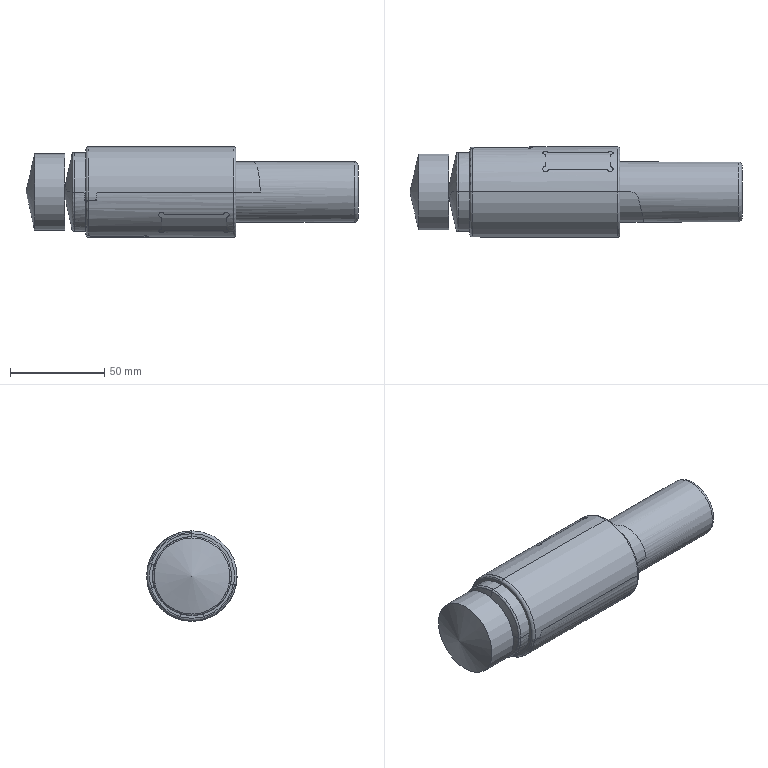Part | 6 solids | 213 faces | box 176.413 x 48 x 48 mm | volume 547716 mm3 | cylinder 94 | plane 93 | torus 15 | cone 11 | commonest cylinder face diameters 3 x48 3.3 x12 2 x4 2.12 x4 32 x3 42 x3